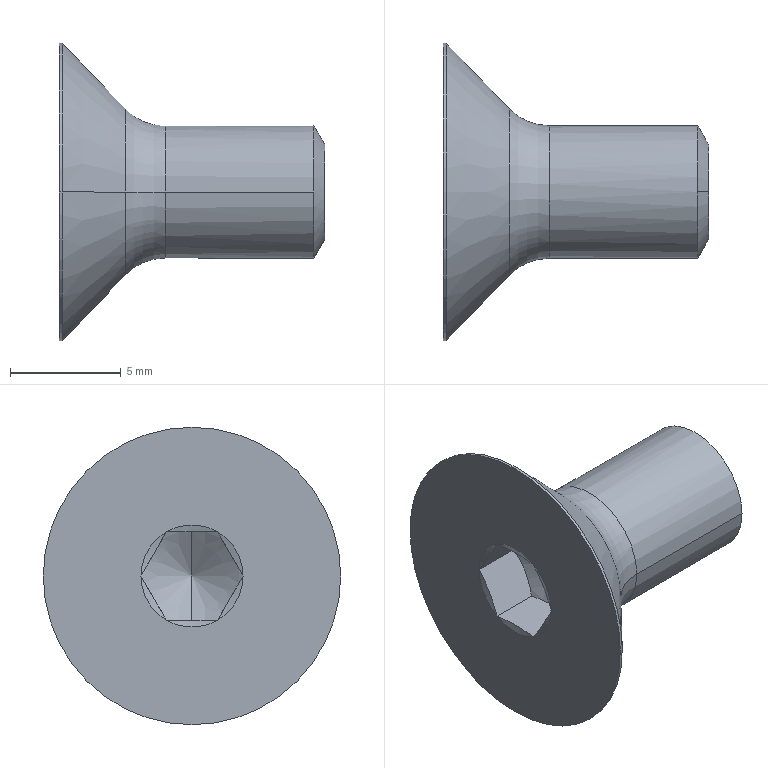Part | SolidWorks | features RevCut 2, Revolution 2, Cut 1, LPattern 1, RefAxis 1 | 1 solid | 26 faces | box 12 x 13.44 x 13.44 mm | volume 493.143 mm3 | cone 12 | plane 8 | cylinder 4 | torus 2 | commonest cylinder face diameters 6 x2 13.44 x2
STEP:
#1=CARTESIAN_POINT('',(0.,0.,2.134));
#2=VERTEX_POINT('',#1);
#3=CARTESIAN_POINT('',(0.,0.,-2.134));
#4=VERTEX_POINT('',#3);
#5=CARTESIAN_POINT('',(0.,0.,0.));
#6=DIRECTION('',(-1.,0.,0.));
#7=DIRECTION('',(0.,0.,1.));
#8=AXIS2_PLACEMENT_3D('',#5,#6,#7);
#9=CIRCLE('',#8,2.134);
#10=EDGE_CURVE('',#2,#4,#9,.T.);
#11=ORIENTED_EDGE('',*,*,#10,.T.);
#12=CARTESIAN_POINT('',(-0.5,0.,-3.));
#13=VERTEX_POINT('',#12);
#14=CARTESIAN_POINT('',(-0.5,0.,-3.));
#15=DIRECTION('',(-0.5,0.,-0.866));
#16=VECTOR('',#15,1000.);
#17=LINE('',#14,#16);
#18=EDGE_CURVE('',#4,#13,#17,.T.);
#19=ORIENTED_EDGE('',*,*,#18,.T.);
#20=CARTESIAN_POINT('',(-0.5,3.,0.));
#21=VERTEX_POINT('',#20);
#22=CARTESIAN_POINT('',(-0.5,0.,0.));
#23=DIRECTION('',(-1.,0.,0.));
#24=DIRECTION('',(0.,0.,1.));
#25=AXIS2_PLACEMENT_3D('',#22,#23,#24);
#26=CIRCLE('',#25,3.);
#27=EDGE_CURVE('',#21,#13,#26,.T.);
#28=ORIENTED_EDGE('',*,*,#27,.F.);
#29=CARTESIAN_POINT('',(-0.5,0.,3.));
#30=VERTEX_POINT('',#29);
#31=CARTESIAN_POINT('',(-0.5,0.,0.));
#32=DIRECTION('',(-1.,0.,0.));
#33=DIRECTION('',(0.,0.,1.));
#34=AXIS2_PLACEMENT_3D('',#31,#32,#33);
#35=CIRCLE('',#34,3.);
#36=EDGE_CURVE('',#30,#21,#35,.T.);
#37=ORIENTED_EDGE('',*,*,#36,.F.);
#38=CARTESIAN_POINT('',(-0.5,0.,3.));
#39=DIRECTION('',(-0.5,0.,0.866));
#40=VECTOR('',#39,1000.);
#41=LINE('',#38,#40);
#42=EDGE_CURVE('',#2,#30,#41,.T.);
#43=ORIENTED_EDGE('',*,*,#42,.F.);
#44=EDGE_LOOP('',(#11,#19,#28,#37,#43));
#45=FACE_OUTER_BOUND('',#44,.T.);
#46=CARTESIAN_POINT('',(-0.5,0.,0.));
#47=DIRECTION('',(-1.,0.,0.));
#48=DIRECTION('',(0.,0.,1.));
#49=AXIS2_PLACEMENT_3D('',#46,#47,#48);
#50=CONICAL_SURFACE('',#49,3.,1.047);
#51=ADVANCED_FACE('',(#45),#50,.T.);
#52=CARTESIAN_POINT('',(-8.467,0.,0.));
#53=VERTEX_POINT('',#52);
#54=CARTESIAN_POINT('',(-9.621,0.,2.));
#55=VERTEX_POINT('',#54);
#56=CARTESIAN_POINT('',(-9.8,0.,2.309));
#57=DIRECTION('',(-0.5,0.,0.866));
#58=VECTOR('',#57,1000.);
#59=LINE('',#56,#58);
#60=EDGE_CURVE('',#53,#55,#59,.T.);
#61=ORIENTED_EDGE('',*,*,#60,.F.);
#62=CARTESIAN_POINT('',(-9.621,0.,-2.));
#63=VERTEX_POINT('',#62);
#64=CARTESIAN_POINT('',(-9.8,0.,-2.309));
#65=DIRECTION('',(-0.5,0.,-0.866));
#66=VECTOR('',#65,1000.);
#67=LINE('',#64,#66);
#68=EDGE_CURVE('',#53,#63,#67,.T.);
#69=ORIENTED_EDGE('',*,*,#68,.T.);
#70=CARTESIAN_POINT('',(-9.8,-1.155,-2.));
#71=VERTEX_POINT('',#70);
#72=CARTESIAN_POINT('',(-9.621,0.,-2.));
#73=CARTESIAN_POINT('',(-9.621,-0.1949,-2.));
#74=CARTESIAN_POINT('',(-9.638,-0.3888,-2.));
#75=CARTESIAN_POINT('',(-9.7,-0.7748,-2.));
#76=CARTESIAN_POINT('',(-9.746,-0.9671,-2.));
#77=CARTESIAN_POINT('',(-9.8,-1.155,-2.));
#78=B_SPLINE_CURVE_WITH_KNOTS('',3,(#72,#73,#74,#75,#76,#77),.UNSPECIFIED.,.F.,.F.,(4,2,4),(0.007354,0.007938,0.008523),.UNSPECIFIED.);
#79=EDGE_CURVE('',#63,#71,#78,.T.);
#80=ORIENTED_EDGE('',*,*,#79,.T.);
#81=CARTESIAN_POINT('',(-9.8,-2.309,0.));
#82=VERTEX_POINT('',#81);
#83=CARTESIAN_POINT('',(-9.8,-1.155,-2.));
#84=CARTESIAN_POINT('',(-9.691,-1.343,-1.673));
#85=CARTESIAN_POINT('',(-9.622,-1.535,-1.342));
#86=CARTESIAN_POINT('',(-9.621,-1.829,-0.8319));
#87=CARTESIAN_POINT('',(-9.638,-1.927,-0.662));
#88=CARTESIAN_POINT('',(-9.701,-2.12,-0.3283));
#89=CARTESIAN_POINT('',(-9.746,-2.215,-0.1635));
#90=CARTESIAN_POINT('',(-9.8,-2.309,0.));
#91=B_SPLINE_CURVE_WITH_KNOTS('',3,(#83,#84,#85,#86,#87,#88,#89,#90),.UNSPECIFIED.,.F.,.F.,(4,2,2,4),(0.000000238,0.001166,0.00175,0.002333),.UNSPECIFIED.);
#92=EDGE_CURVE('',#71,#82,#91,.T.);
#93=ORIENTED_EDGE('',*,*,#92,.T.);
#94=CARTESIAN_POINT('',(-9.8,-1.155,2.));
#95=VERTEX_POINT('',#94);
#96=CARTESIAN_POINT('',(-9.8,-2.309,0.));
#97=CARTESIAN_POINT('',(-9.691,-2.121,0.3266));
#98=CARTESIAN_POINT('',(-9.622,-1.929,0.658));
#99=CARTESIAN_POINT('',(-9.621,-1.635,1.168));
#100=CARTESIAN_POINT('',(-9.638,-1.537,1.338));
#101=CARTESIAN_POINT('',(-9.701,-1.344,1.672));
#102=CARTESIAN_POINT('',(-9.746,-1.249,1.837));
#103=CARTESIAN_POINT('',(-9.8,-1.155,2.));
#104=B_SPLINE_CURVE_WITH_KNOTS('',3,(#96,#97,#98,#99,#100,#101,#102,#103),.UNSPECIFIED.,.F.,.F.,(4,2,2,4),(0.000000238,0.001166,0.00175,0.002333),.UNSPECIFIED.);
#105=EDGE_CURVE('',#82,#95,#104,.T.);
#106=ORIENTED_EDGE('',*,*,#105,.T.);
#107=CARTESIAN_POINT('',(-9.8,-1.155,2.));
#108=CARTESIAN_POINT('',(-9.746,-0.9671,2.));
#109=CARTESIAN_POINT('',(-9.7,-0.7748,2.));
#110=CARTESIAN_POINT('',(-9.638,-0.3888,2.));
#111=CARTESIAN_POINT('',(-9.621,-0.1949,2.));
#112=CARTESIAN_POINT('',(-9.621,0.,2.));
#113=B_SPLINE_CURVE_WITH_KNOTS('',3,(#107,#108,#109,#110,#111,#112),.UNSPECIFIED.,.F.,.F.,(4,2,4),(0.00198,0.002564,0.003147),.UNSPECIFIED.);
#114=EDGE_CURVE('',#95,#55,#113,.T.);
#115=ORIENTED_EDGE('',*,*,#114,.T.);
#116=EDGE_LOOP('',(#61,#69,#80,#93,#106,#115));
#117=FACE_OUTER_BOUND('',#116,.T.);
#118=CARTESIAN_POINT('',(-9.8,0.,0.));
#119=DIRECTION('',(-1.,0.,0.));
#120=DIRECTION('',(0.,0.,1.));
#121=AXIS2_PLACEMENT_3D('',#118,#119,#120);
#122=CONICAL_SURFACE('',#121,2.309,1.047);
#123=ADVANCED_FACE('',(#117),#122,.F.);
#124=CARTESIAN_POINT('',(-7.219,-3.,0.));
#125=VERTEX_POINT('',#124);
#126=CARTESIAN_POINT('',(-7.219,3.,0.));
#127=VERTEX_POINT('',#126);
#128=CARTESIAN_POINT('',(-7.219,0.,0.));
#129=DIRECTION('',(1.,0.,0.));
#130=DIRECTION('',(0.,1.,0.));
#131=AXIS2_PLACEMENT_3D('',#128,#129,#130);
#132=CIRCLE('',#131,3.);
#133=EDGE_CURVE('',#125,#127,#132,.T.);
#134=ORIENTED_EDGE('',*,*,#133,.F.);
#135=CARTESIAN_POINT('',(-9.017,-3.763,0.));
#136=VERTEX_POINT('',#135);
#137=CARTESIAN_POINT('',(-7.219,-5.5,0.));
#138=DIRECTION('',(0.,0.,1.));
#139=DIRECTION('',(0.,-1.,0.));
#140=AXIS2_PLACEMENT_3D('',#137,#138,#139);
#141=CIRCLE('',#140,2.5);
#142=EDGE_CURVE('',#125,#136,#141,.T.);
#143=ORIENTED_EDGE('',*,*,#142,.T.);
#144=CARTESIAN_POINT('',(-9.017,3.763,0.));
#145=VERTEX_POINT('',#144);
#146=CARTESIAN_POINT('',(-9.017,0.,0.));
#147=DIRECTION('',(1.,0.,0.));
#148=DIRECTION('',(0.,1.,0.));
#149=AXIS2_PLACEMENT_3D('',#146,#147,#148);
#150=CIRCLE('',#149,3.763);
#151=EDGE_CURVE('',#136,#145,#150,.T.);
#152=ORIENTED_EDGE('',*,*,#151,.T.);
#153=CARTESIAN_POINT('',(-7.219,5.5,0.));
#154=DIRECTION('',(0.,0.,-1.));
#155=DIRECTION('',(-1.,0.,0.));
#156=AXIS2_PLACEMENT_3D('',#153,#154,#155);
#157=CIRCLE('',#156,2.5);
#158=EDGE_CURVE('',#127,#145,#157,.T.);
#159=ORIENTED_EDGE('',*,*,#158,.F.);
#160=EDGE_LOOP('',(#134,#143,#152,#159));
#161=FACE_OUTER_BOUND('',#160,.T.);
#162=CARTESIAN_POINT('',(-7.219,0.,0.));
#163=DIRECTION('',(1.,0.,0.));
#164=DIRECTION('',(0.,1.,0.));
#165=AXIS2_PLACEMENT_3D('',#162,#163,#164);
#166=TOROIDAL_SURFACE('',#165,5.5,2.5);
#167=ADVANCED_FACE('',(#161),#166,.F.);
#168=CARTESIAN_POINT('',(-9.017,0.,0.));
#169=DIRECTION('',(1.,0.,0.));
#170=DIRECTION('',(0.,1.,0.));
#171=AXIS2_PLACEMENT_3D('',#168,#169,#170);
#172=CIRCLE('',#171,3.763);
#173=EDGE_CURVE('',#145,#136,#172,.T.);
#174=ORIENTED_EDGE('',*,*,#173,.F.);
#175=CARTESIAN_POINT('',(-11.872,6.72,0.));
#176=VERTEX_POINT('',#175);
#177=CARTESIAN_POINT('',(-9.017,3.763,0.));
#178=DIRECTION('',(-0.6947,0.7193,0.));
#179=VECTOR('',#178,1000.);
#180=LINE('',#177,#179);
#181=EDGE_CURVE('',#145,#176,#180,.T.);
#182=ORIENTED_EDGE('',*,*,#181,.T.);
#183=CARTESIAN_POINT('',(-11.872,-6.72,0.));
#184=VERTEX_POINT('',#183);
#185=CARTESIAN_POINT('',(-11.872,0.,0.));
#186=DIRECTION('',(1.,0.,0.));
#187=DIRECTION('',(0.,1.,0.));
#188=AXIS2_PLACEMENT_3D('',#185,#186,#187);
#189=CIRCLE('',#188,6.72);
#190=EDGE_CURVE('',#176,#184,#189,.T.);
#191=ORIENTED_EDGE('',*,*,#190,.T.);
#192=CARTESIAN_POINT('',(-9.017,-3.763,0.));
#193=DIRECTION('',(-0.6947,-0.7193,0.));
#194=VECTOR('',#193,1000.);
#195=LINE('',#192,#194);
#196=EDGE_CURVE('',#136,#184,#195,.T.);
#197=ORIENTED_EDGE('',*,*,#196,.F.);
#198=EDGE_LOOP('',(#174,#182,#191,#197));
#199=FACE_OUTER_BOUND('',#198,.T.);
#200=CARTESIAN_POINT('',(-9.017,0.,0.));
#201=DIRECTION('',(-1.,0.,0.));
#202=DIRECTION('',(0.,-1.,0.));
#203=AXIS2_PLACEMENT_3D('',#200,#201,#202);
#204=CONICAL_SURFACE('',#203,3.763,0.8029);
#205=ADVANCED_FACE('',(#199),#204,.T.);
#206=CARTESIAN_POINT('',(-12.,6.72,0.));
#207=VERTEX_POINT('',#206);
#208=CARTESIAN_POINT('',(-12.,-6.72,0.));
#209=VERTEX_POINT('',#208);
#210=CARTESIAN_POINT('',(-12.,0.,0.));
#211=DIRECTION('',(1.,0.,0.));
#212=DIRECTION('',(0.,1.,0.));
#213=AXIS2_PLACEMENT_3D('',#210,#211,#212);
#214=CIRCLE('',#213,6.72);
#215=EDGE_CURVE('',#207,#209,#214,.T.);
#216=ORIENTED_EDGE('',*,*,#215,.T.);
#217=CARTESIAN_POINT('',(0.,-6.72,0.));
#218=DIRECTION('',(1.,0.,0.));
#219=VECTOR('',#218,1000.);
#220=LINE('',#217,#219);
#221=EDGE_CURVE('',#209,#184,#220,.T.);
#222=ORIENTED_EDGE('',*,*,#221,.T.);
#223=ORIENTED_EDGE('',*,*,#190,.F.);
#224=CARTESIAN_POINT('',(0.,6.72,0.));
#225=DIRECTION('',(1.,0.,0.));
#226=VECTOR('',#225,1000.);
#227=LINE('',#224,#226);
#228=EDGE_CURVE('',#207,#176,#227,.T.);
#229=ORIENTED_EDGE('',*,*,#228,.F.);
#230=EDGE_LOOP('',(#216,#222,#223,#229));
#231=FACE_OUTER_BOUND('',#230,.T.);
#232=CARTESIAN_POINT('',(0.,0.,0.));
#233=DIRECTION('',(1.,0.,0.));
#234=DIRECTION('',(0.,1.,0.));
#235=AXIS2_PLACEMENT_3D('',#232,#233,#234);
#236=CYLINDRICAL_SURFACE('',#235,6.72);
#237=ADVANCED_FACE('',(#231),#236,.T.);
#238=CARTESIAN_POINT('',(-7.219,0.,0.));
#239=DIRECTION('',(1.,0.,0.));
#240=DIRECTION('',(0.,1.,0.));
#241=AXIS2_PLACEMENT_3D('',#238,#239,#240);
#242=CIRCLE('',#241,3.);
#243=EDGE_CURVE('',#127,#125,#242,.T.);
#244=ORIENTED_EDGE('',*,*,#243,.T.);
#245=CARTESIAN_POINT('',(-0.5,-3.,0.));
#246=VERTEX_POINT('',#245);
#247=CARTESIAN_POINT('',(0.,-3.,0.));
#248=DIRECTION('',(1.,0.,0.));
#249=VECTOR('',#248,1000.);
#250=LINE('',#247,#249);
#251=EDGE_CURVE('',#125,#246,#250,.T.);
#252=ORIENTED_EDGE('',*,*,#251,.T.);
#253=CARTESIAN_POINT('',(-0.5,0.,0.));
#254=DIRECTION('',(-1.,0.,0.));
#255=DIRECTION('',(0.,0.,1.));
#256=AXIS2_PLACEMENT_3D('',#253,#254,#255);
#257=CIRCLE('',#256,3.);
#258=EDGE_CURVE('',#246,#30,#257,.T.);
#259=ORIENTED_EDGE('',*,*,#258,.T.);
#260=ORIENTED_EDGE('',*,*,#36,.T.);
#261=CARTESIAN_POINT('',(0.,3.,0.));
#262=DIRECTION('',(1.,0.,0.));
#263=VECTOR('',#262,1000.);
#264=LINE('',#261,#263);
#265=EDGE_CURVE('',#127,#21,#264,.T.);
#266=ORIENTED_EDGE('',*,*,#265,.F.);
#267=EDGE_LOOP('',(#244,#252,#259,#260,#266));
#268=FACE_OUTER_BOUND('',#267,.T.);
#269=CARTESIAN_POINT('',(0.,0.,0.));
#270=DIRECTION('',(1.,0.,0.));
#271=DIRECTION('',(0.,1.,0.));
#272=AXIS2_PLACEMENT_3D('',#269,#270,#271);
#273=CYLINDRICAL_SURFACE('',#272,3.);
#274=ADVANCED_FACE('',(#268),#273,.T.);
#275=ORIENTED_EDGE('',*,*,#251,.F.);
#276=ORIENTED_EDGE('',*,*,#133,.T.);
#277=ORIENTED_EDGE('',*,*,#265,.T.);
#278=ORIENTED_EDGE('',*,*,#27,.T.);
#279=CARTESIAN_POINT('',(-0.5,0.,0.));
#280=DIRECTION('',(-1.,0.,0.));
#281=DIRECTION('',(0.,0.,1.));
#282=AXIS2_PLACEMENT_3D('',#279,#280,#281);
#283=CIRCLE('',#282,3.);
#284=EDGE_CURVE('',#13,#246,#283,.T.);
#285=ORIENTED_EDGE('',*,*,#284,.T.);
#286=EDGE_LOOP('',(#275,#276,#277,#278,#285));
#287=FACE_OUTER_BOUND('',#286,.T.);
#288=CARTESIAN_POINT('',(0.,0.,0.));
#289=DIRECTION('',(1.,0.,0.));
#290=DIRECTION('',(0.,1.,0.));
#291=AXIS2_PLACEMENT_3D('',#288,#289,#290);
#292=CYLINDRICAL_SURFACE('',#291,3.);
#293=ADVANCED_FACE('',(#287),#292,.T.);
#294=ORIENTED_EDGE('',*,*,#215,.F.);
#295=CARTESIAN_POINT('',(-12.,0.,0.));
#296=DIRECTION('',(1.,0.,0.));
#297=DIRECTION('',(0.,1.,0.));
#298=AXIS2_PLACEMENT_3D('',#295,#296,#297);
#299=CIRCLE('',#298,6.72);
#300=EDGE_CURVE('',#209,#207,#299,.T.);
#301=ORIENTED_EDGE('',*,*,#300,.F.);
#302=EDGE_LOOP('',(#294,#301));
#303=FACE_OUTER_BOUND('',#302,.T.);
#304=CARTESIAN_POINT('',(-12.,-2.309,0.));
#305=VERTEX_POINT('',#304);
#306=CARTESIAN_POINT('',(-12.,-1.155,2.));
#307=VERTEX_POINT('',#306);
#308=CARTESIAN_POINT('',(-12.,0.,0.));
#309=DIRECTION('',(-1.,0.,0.));
#310=DIRECTION('',(0.,-1.,0.));
#311=AXIS2_PLACEMENT_3D('',#308,#309,#310);
#312=CIRCLE('',#311,2.309);
#313=EDGE_CURVE('',#305,#307,#312,.T.);
#314=ORIENTED_EDGE('',*,*,#313,.F.);
#315=CARTESIAN_POINT('',(-12.,-1.155,-2.));
#316=VERTEX_POINT('',#315);
#317=CARTESIAN_POINT('',(-12.,0.,0.));
#318=DIRECTION('',(1.,0.,0.));
#319=DIRECTION('',(0.,-1.,0.));
#320=AXIS2_PLACEMENT_3D('',#317,#318,#319);
#321=CIRCLE('',#320,2.309);
#322=EDGE_CURVE('',#305,#316,#321,.T.);
#323=ORIENTED_EDGE('',*,*,#322,.T.);
#324=CARTESIAN_POINT('',(-12.,1.155,-2.));
#325=VERTEX_POINT('',#324);
#326=CARTESIAN_POINT('',(-12.,0.,0.));
#327=DIRECTION('',(1.,0.,0.));
#328=DIRECTION('',(0.,-1.,0.));
#329=AXIS2_PLACEMENT_3D('',#326,#327,#328);
#330=CIRCLE('',#329,2.309);
#331=EDGE_CURVE('',#316,#325,#330,.T.);
#332=ORIENTED_EDGE('',*,*,#331,.T.);
#333=CARTESIAN_POINT('',(-12.,2.309,0.));
#334=VERTEX_POINT('',#333);
#335=CARTESIAN_POINT('',(-12.,0.,0.));
#336=DIRECTION('',(1.,0.,0.));
#337=DIRECTION('',(0.,-1.,0.));
#338=AXIS2_PLACEMENT_3D('',#335,#336,#337);
#339=CIRCLE('',#338,2.309);
#340=EDGE_CURVE('',#325,#334,#339,.T.);
#341=ORIENTED_EDGE('',*,*,#340,.T.);
#342=CARTESIAN_POINT('',(-12.,1.155,2.));
#343=VERTEX_POINT('',#342);
#344=CARTESIAN_POINT('',(-12.,0.,0.));
#345=DIRECTION('',(1.,0.,0.));
#346=DIRECTION('',(0.,-1.,0.));
#347=AXIS2_PLACEMENT_3D('',#344,#345,#346);
#348=CIRCLE('',#347,2.309);
#349=EDGE_CURVE('',#334,#343,#348,.T.);
#350=ORIENTED_EDGE('',*,*,#349,.T.);
#351=CARTESIAN_POINT('',(-12.,0.,0.));
#352=DIRECTION('',(1.,0.,0.));
#353=DIRECTION('',(0.,-1.,0.));
#354=AXIS2_PLACEMENT_3D('',#351,#352,#353);
#355=CIRCLE('',#354,2.309);
#356=EDGE_CURVE('',#343,#307,#355,.T.);
#357=ORIENTED_EDGE('',*,*,#356,.T.);
#358=EDGE_LOOP('',(#314,#323,#332,#341,#350,#357));
#359=FACE_BOUND('',#358,.T.);
#360=CARTESIAN_POINT('',(-12.,6.72,0.));
#361=DIRECTION('',(-1.,0.,0.));
#362=DIRECTION('',(0.,-1.,0.));
#363=AXIS2_PLACEMENT_3D('',#360,#361,#362);
#364=PLANE('',#363);
#365=ADVANCED_FACE('',(#303,#359),#364,.T.);
#366=ORIENTED_EDGE('',*,*,#221,.F.);
#367=ORIENTED_EDGE('',*,*,#300,.T.);
#368=ORIENTED_EDGE('',*,*,#228,.T.);
#369=CARTESIAN_POINT('',(-11.872,0.,0.));
#370=DIRECTION('',(1.,0.,0.));
#371=DIRECTION('',(0.,1.,0.));
#372=AXIS2_PLACEMENT_3D('',#369,#370,#371);
#373=CIRCLE('',#372,6.72);
#374=EDGE_CURVE('',#184,#176,#373,.T.);
#375=ORIENTED_EDGE('',*,*,#374,.F.);
#376=EDGE_LOOP('',(#366,#367,#368,#375));
#377=FACE_OUTER_BOUND('',#376,.T.);
#378=CARTESIAN_POINT('',(0.,0.,0.));
#379=DIRECTION('',(1.,0.,0.));
#380=DIRECTION('',(0.,1.,0.));
#381=AXIS2_PLACEMENT_3D('',#378,#379,#380);
#382=CYLINDRICAL_SURFACE('',#381,6.72);
#383=ADVANCED_FACE('',(#377),#382,.T.);
#384=ORIENTED_EDGE('',*,*,#181,.F.);
#385=ORIENTED_EDGE('',*,*,#151,.F.);
#386=ORIENTED_EDGE('',*,*,#196,.T.);
#387=ORIENTED_EDGE('',*,*,#374,.T.);
#388=EDGE_LOOP('',(#384,#385,#386,#387));
#389=FACE_OUTER_BOUND('',#388,.T.);
#390=CARTESIAN_POINT('',(-9.017,0.,0.));
#391=DIRECTION('',(-1.,0.,0.));
#392=DIRECTION('',(0.,-1.,0.));
#393=AXIS2_PLACEMENT_3D('',#390,#391,#392);
#394=CONICAL_SURFACE('',#393,3.763,0.8029);
#395=ADVANCED_FACE('',(#389),#394,.T.);
#396=ORIENTED_EDGE('',*,*,#142,.F.);
#397=ORIENTED_EDGE('',*,*,#243,.F.);
#398=ORIENTED_EDGE('',*,*,#158,.T.);
#399=ORIENTED_EDGE('',*,*,#173,.T.);
#400=EDGE_LOOP('',(#396,#397,#398,#399));
#401=FACE_OUTER_BOUND('',#400,.T.);
#402=CARTESIAN_POINT('',(-7.219,0.,0.));
#403=DIRECTION('',(1.,0.,0.));
#404=DIRECTION('',(0.,1.,0.));
#405=AXIS2_PLACEMENT_3D('',#402,#403,#404);
#406=TOROIDAL_SURFACE('',#405,5.5,2.5);
#407=ADVANCED_FACE('',(#401),#406,.F.);
#408=CARTESIAN_POINT('',(-12.,-1.155,2.));
#409=CARTESIAN_POINT('',(-11.947,-1.347,1.667));
#410=CARTESIAN_POINT('',(-11.882,-1.732,1.));
#411=CARTESIAN_POINT('',(-11.947,-2.117,0.3333));
#412=CARTESIAN_POINT('',(-12.,-2.309,0.));
#413=B_SPLINE_CURVE_WITH_KNOTS('',3,(#408,#409,#410,#411,#412),.UNSPECIFIED.,.F.,.F.,(4,1,4),(0.000000231,0.001155,0.00231),.UNSPECIFIED.);
#414=EDGE_CURVE('',#307,#305,#413,.T.);
#415=ORIENTED_EDGE('',*,*,#414,.T.);
#416=ORIENTED_EDGE('',*,*,#313,.T.);
#417=EDGE_LOOP('',(#415,#416));
#418=FACE_OUTER_BOUND('',#417,.T.);
#419=CARTESIAN_POINT('',(-1011.362,0.,0.));
#420=DIRECTION('',(-1.,0.,0.));
#421=DIRECTION('',(0.,-1.,0.));
#422=AXIS2_PLACEMENT_3D('',#419,#420,#421);
#423=CONICAL_SURFACE('',#422,3619.751,1.301);
#424=ADVANCED_FACE('',(#418),#423,.F.);
#425=CARTESIAN_POINT('',(-12.,1.155,2.));
#426=CARTESIAN_POINT('',(-11.947,0.7714,2.));
#427=CARTESIAN_POINT('',(-11.915,0.3874,2.));
#428=CARTESIAN_POINT('',(-11.914,-0.3828,2.));
#429=CARTESIAN_POINT('',(-11.947,-0.7704,2.));
#430=CARTESIAN_POINT('',(-12.,-1.155,2.));
#431=B_SPLINE_CURVE_WITH_KNOTS('',3,(#425,#426,#427,#428,#429,#430),.UNSPECIFIED.,.F.,.F.,(4,2,4),(0.004828,0.005989,0.007149),.UNSPECIFIED.);
#432=EDGE_CURVE('',#343,#307,#431,.T.);
#433=ORIENTED_EDGE('',*,*,#432,.T.);
#434=ORIENTED_EDGE('',*,*,#356,.F.);
#435=EDGE_LOOP('',(#433,#434));
#436=FACE_OUTER_BOUND('',#435,.T.);
#437=CARTESIAN_POINT('',(-1011.362,0.,0.));
#438=DIRECTION('',(-1.,0.,0.));
#439=DIRECTION('',(0.,-1.,0.));
#440=AXIS2_PLACEMENT_3D('',#437,#438,#439);
#441=CONICAL_SURFACE('',#440,3619.751,1.301);
#442=ADVANCED_FACE('',(#436),#441,.F.);
#443=CARTESIAN_POINT('',(-12.,2.309,0.));
#444=CARTESIAN_POINT('',(-11.947,2.117,0.3333));
#445=CARTESIAN_POINT('',(-11.882,1.732,1.));
#446=CARTESIAN_POINT('',(-11.947,1.347,1.667));
#447=CARTESIAN_POINT('',(-12.,1.155,2.));
#448=B_SPLINE_CURVE_WITH_KNOTS('',3,(#443,#444,#445,#446,#447),.UNSPECIFIED.,.F.,.F.,(4,1,4),(0.000000231,0.001155,0.00231),.UNSPECIFIED.);
#449=EDGE_CURVE('',#334,#343,#448,.T.);
#450=ORIENTED_EDGE('',*,*,#449,.T.);
#451=ORIENTED_EDGE('',*,*,#349,.F.);
#452=EDGE_LOOP('',(#450,#451));
#453=FACE_OUTER_BOUND('',#452,.T.);
#454=CARTESIAN_POINT('',(-1011.362,0.,0.));
#455=DIRECTION('',(-1.,0.,0.));
#456=DIRECTION('',(0.,-1.,0.));
#457=AXIS2_PLACEMENT_3D('',#454,#455,#456);
#458=CONICAL_SURFACE('',#457,3619.751,1.301);
#459=ADVANCED_FACE('',(#453),#458,.F.);
#460=CARTESIAN_POINT('',(-12.,1.155,-2.));
#461=CARTESIAN_POINT('',(-11.947,1.347,-1.667));
#462=CARTESIAN_POINT('',(-11.882,1.732,-1.));
#463=CARTESIAN_POINT('',(-11.947,2.117,-0.3333));
#464=CARTESIAN_POINT('',(-12.,2.309,0.));
#465=B_SPLINE_CURVE_WITH_KNOTS('',3,(#460,#461,#462,#463,#464),.UNSPECIFIED.,.F.,.F.,(4,1,4),(0.000000231,0.001155,0.00231),.UNSPECIFIED.);
#466=EDGE_CURVE('',#325,#334,#465,.T.);
#467=ORIENTED_EDGE('',*,*,#466,.T.);
#468=ORIENTED_EDGE('',*,*,#340,.F.);
#469=EDGE_LOOP('',(#467,#468));
#470=FACE_OUTER_BOUND('',#469,.T.);
#471=CARTESIAN_POINT('',(-1011.362,0.,0.));
#472=DIRECTION('',(-1.,0.,0.));
#473=DIRECTION('',(0.,-1.,0.));
#474=AXIS2_PLACEMENT_3D('',#471,#472,#473);
#475=CONICAL_SURFACE('',#474,3619.751,1.301);
#476=ADVANCED_FACE('',(#470),#475,.F.);
#477=CARTESIAN_POINT('',(-12.,-1.155,-2.));
#478=CARTESIAN_POINT('',(-11.947,-0.7704,-2.));
#479=CARTESIAN_POINT('',(-11.914,-0.3828,-2.));
#480=CARTESIAN_POINT('',(-11.915,0.3874,-2.));
#481=CARTESIAN_POINT('',(-11.947,0.7714,-2.));
#482=CARTESIAN_POINT('',(-12.,1.155,-2.));
#483=B_SPLINE_CURVE_WITH_KNOTS('',3,(#477,#478,#479,#480,#481,#482),.UNSPECIFIED.,.F.,.F.,(4,2,4),(0.001892,0.003055,0.004218),.UNSPECIFIED.);
#484=EDGE_CURVE('',#316,#325,#483,.T.);
#485=ORIENTED_EDGE('',*,*,#484,.T.);
#486=ORIENTED_EDGE('',*,*,#331,.F.);
#487=EDGE_LOOP('',(#485,#486));
#488=FACE_OUTER_BOUND('',#487,.T.);
#489=CARTESIAN_POINT('',(-1011.362,0.,0.));
#490=DIRECTION('',(-1.,0.,0.));
#491=DIRECTION('',(0.,-1.,0.));
#492=AXIS2_PLACEMENT_3D('',#489,#490,#491);
#493=CONICAL_SURFACE('',#492,3619.751,1.301);
#494=ADVANCED_FACE('',(#488),#493,.F.);
#495=CARTESIAN_POINT('',(-12.,-2.309,0.));
#496=CARTESIAN_POINT('',(-11.947,-2.117,-0.3333));
#497=CARTESIAN_POINT('',(-11.882,-1.732,-1.));
#498=CARTESIAN_POINT('',(-11.947,-1.347,-1.667));
#499=CARTESIAN_POINT('',(-12.,-1.155,-2.));
#500=B_SPLINE_CURVE_WITH_KNOTS('',3,(#495,#496,#497,#498,#499),.UNSPECIFIED.,.F.,.F.,(4,1,4),(0.000000231,0.001155,0.00231),.UNSPECIFIED.);
#501=EDGE_CURVE('',#305,#316,#500,.T.);
#502=ORIENTED_EDGE('',*,*,#501,.T.);
#503=ORIENTED_EDGE('',*,*,#322,.F.);
#504=EDGE_LOOP('',(#502,#503));
#505=FACE_OUTER_BOUND('',#504,.T.);
#506=CARTESIAN_POINT('',(-1011.362,0.,0.));
#507=DIRECTION('',(-1.,0.,0.));
#508=DIRECTION('',(0.,-1.,0.));
#509=AXIS2_PLACEMENT_3D('',#506,#507,#508);
#510=CONICAL_SURFACE('',#509,3619.751,1.301);
#511=ADVANCED_FACE('',(#505),#510,.F.);
#512=ORIENTED_EDGE('',*,*,#68,.F.);
#513=ORIENTED_EDGE('',*,*,#60,.T.);
#514=CARTESIAN_POINT('',(-9.8,1.155,2.));
#515=VERTEX_POINT('',#514);
#516=CARTESIAN_POINT('',(-9.621,0.,2.));
#517=CARTESIAN_POINT('',(-9.621,0.195,2.));
#518=CARTESIAN_POINT('',(-9.639,0.3927,2.));
#519=CARTESIAN_POINT('',(-9.701,0.7788,2.));
#520=CARTESIAN_POINT('',(-9.746,0.968,2.));
#521=CARTESIAN_POINT('',(-9.8,1.155,2.));
#522=B_SPLINE_CURVE_WITH_KNOTS('',3,(#516,#517,#518,#519,#520,#521),.UNSPECIFIED.,.F.,.F.,(4,2,4),(0.003147,0.003731,0.004315),.UNSPECIFIED.);
#523=EDGE_CURVE('',#55,#515,#522,.T.);
#524=ORIENTED_EDGE('',*,*,#523,.T.);
#525=CARTESIAN_POINT('',(-9.8,2.309,0.));
#526=VERTEX_POINT('',#525);
#527=CARTESIAN_POINT('',(-9.8,1.155,2.));
#528=CARTESIAN_POINT('',(-9.691,1.343,1.673));
#529=CARTESIAN_POINT('',(-9.622,1.535,1.342));
#530=CARTESIAN_POINT('',(-9.621,1.829,0.8319));
#531=CARTESIAN_POINT('',(-9.638,1.927,0.662));
#532=CARTESIAN_POINT('',(-9.701,2.12,0.3283));
#533=CARTESIAN_POINT('',(-9.746,2.215,0.1635));
#534=CARTESIAN_POINT('',(-9.8,2.309,0.));
#535=B_SPLINE_CURVE_WITH_KNOTS('',3,(#527,#528,#529,#530,#531,#532,#533,#534),.UNSPECIFIED.,.F.,.F.,(4,2,2,4),(0.000000238,0.001166,0.00175,0.002333),.UNSPECIFIED.);
#536=EDGE_CURVE('',#515,#526,#535,.T.);
#537=ORIENTED_EDGE('',*,*,#536,.T.);
#538=CARTESIAN_POINT('',(-9.8,1.155,-2.));
#539=VERTEX_POINT('',#538);
#540=CARTESIAN_POINT('',(-9.8,2.309,0.));
#541=CARTESIAN_POINT('',(-9.691,2.121,-0.3266));
#542=CARTESIAN_POINT('',(-9.622,1.929,-0.658));
#543=CARTESIAN_POINT('',(-9.621,1.635,-1.168));
#544=CARTESIAN_POINT('',(-9.638,1.537,-1.338));
#545=CARTESIAN_POINT('',(-9.701,1.344,-1.672));
#546=CARTESIAN_POINT('',(-9.746,1.249,-1.837));
#547=CARTESIAN_POINT('',(-9.8,1.155,-2.));
#548=B_SPLINE_CURVE_WITH_KNOTS('',3,(#540,#541,#542,#543,#544,#545,#546,#547),.UNSPECIFIED.,.F.,.F.,(4,2,2,4),(0.000000238,0.001166,0.00175,0.002333),.UNSPECIFIED.);
#549=EDGE_CURVE('',#526,#539,#548,.T.);
#550=ORIENTED_EDGE('',*,*,#549,.T.);
#551=CARTESIAN_POINT('',(-9.8,1.155,-2.));
#552=CARTESIAN_POINT('',(-9.746,0.968,-2.));
#553=CARTESIAN_POINT('',(-9.701,0.7788,-2.));
#554=CARTESIAN_POINT('',(-9.639,0.3927,-2.));
#555=CARTESIAN_POINT('',(-9.621,0.195,-2.));
#556=CARTESIAN_POINT('',(-9.621,0.,-2.));
#557=B_SPLINE_CURVE_WITH_KNOTS('',3,(#551,#552,#553,#554,#555,#556),.UNSPECIFIED.,.F.,.F.,(4,2,4),(0.006185,0.006769,0.007354),.UNSPECIFIED.);
#558=EDGE_CURVE('',#539,#63,#557,.T.);
#559=ORIENTED_EDGE('',*,*,#558,.T.);
#560=EDGE_LOOP('',(#512,#513,#524,#537,#550,#559));
#561=FACE_OUTER_BOUND('',#560,.T.);
#562=CARTESIAN_POINT('',(-9.8,0.,0.));
#563=DIRECTION('',(-1.,0.,0.));
#564=DIRECTION('',(0.,0.,1.));
#565=AXIS2_PLACEMENT_3D('',#562,#563,#564);
#566=CONICAL_SURFACE('',#565,2.309,1.047);
#567=ADVANCED_FACE('',(#561),#566,.F.);
#568=ORIENTED_EDGE('',*,*,#466,.F.);
#569=CARTESIAN_POINT('',(-8.18,1.155,-2.));
#570=DIRECTION('',(-1.,0.,0.));
#571=VECTOR('',#570,1000.);
#572=LINE('',#569,#571);
#573=EDGE_CURVE('',#539,#325,#572,.T.);
#574=ORIENTED_EDGE('',*,*,#573,.F.);
#575=ORIENTED_EDGE('',*,*,#549,.F.);
#576=CARTESIAN_POINT('',(-8.18,2.309,0.));
#577=DIRECTION('',(-1.,0.,0.));
#578=VECTOR('',#577,1000.);
#579=LINE('',#576,#578);
#580=EDGE_CURVE('',#526,#334,#579,.T.);
#581=ORIENTED_EDGE('',*,*,#580,.T.);
#582=EDGE_LOOP('',(#568,#574,#575,#581));
#583=FACE_OUTER_BOUND('',#582,.T.);
#584=CARTESIAN_POINT('',(-8.18,2.309,0.));
#585=DIRECTION('',(0.,0.866,-0.5));
#586=DIRECTION('',(0.,0.5,0.866));
#587=AXIS2_PLACEMENT_3D('',#584,#585,#586);
#588=PLANE('',#587);
#589=ADVANCED_FACE('',(#583),#588,.F.);
#590=ORIENTED_EDGE('',*,*,#484,.F.);
#591=CARTESIAN_POINT('',(-8.18,-1.155,-2.));
#592=DIRECTION('',(-1.,0.,0.));
#593=VECTOR('',#592,1000.);
#594=LINE('',#591,#593);
#595=EDGE_CURVE('',#71,#316,#594,.T.);
#596=ORIENTED_EDGE('',*,*,#595,.F.);
#597=ORIENTED_EDGE('',*,*,#79,.F.);
#598=ORIENTED_EDGE('',*,*,#558,.F.);
#599=ORIENTED_EDGE('',*,*,#573,.T.);
#600=EDGE_LOOP('',(#590,#596,#597,#598,#599));
#601=FACE_OUTER_BOUND('',#600,.T.);
#602=CARTESIAN_POINT('',(-8.18,1.155,-2.));
#603=DIRECTION('',(0.,0.,-1.));
#604=DIRECTION('',(-1.,0.,0.));
#605=AXIS2_PLACEMENT_3D('',#602,#603,#604);
#606=PLANE('',#605);
#607=ADVANCED_FACE('',(#601),#606,.F.);
#608=ORIENTED_EDGE('',*,*,#501,.F.);
#609=CARTESIAN_POINT('',(-8.18,-2.309,0.));
#610=DIRECTION('',(-1.,0.,0.));
#611=VECTOR('',#610,1000.);
#612=LINE('',#609,#611);
#613=EDGE_CURVE('',#82,#305,#612,.T.);
#614=ORIENTED_EDGE('',*,*,#613,.F.);
#615=ORIENTED_EDGE('',*,*,#92,.F.);
#616=ORIENTED_EDGE('',*,*,#595,.T.);
#617=EDGE_LOOP('',(#608,#614,#615,#616));
#618=FACE_OUTER_BOUND('',#617,.T.);
#619=CARTESIAN_POINT('',(-8.18,-1.155,-2.));
#620=DIRECTION('',(0.,-0.866,-0.5));
#621=DIRECTION('',(0.,0.5,-0.866));
#622=AXIS2_PLACEMENT_3D('',#619,#620,#621);
#623=PLANE('',#622);
#624=ADVANCED_FACE('',(#618),#623,.F.);
#625=ORIENTED_EDGE('',*,*,#414,.F.);
#626=CARTESIAN_POINT('',(-8.18,-1.155,2.));
#627=DIRECTION('',(-1.,0.,0.));
#628=VECTOR('',#627,1000.);
#629=LINE('',#626,#628);
#630=EDGE_CURVE('',#95,#307,#629,.T.);
#631=ORIENTED_EDGE('',*,*,#630,.F.);
#632=ORIENTED_EDGE('',*,*,#105,.F.);
#633=ORIENTED_EDGE('',*,*,#613,.T.);
#634=EDGE_LOOP('',(#625,#631,#632,#633));
#635=FACE_OUTER_BOUND('',#634,.T.);
#636=CARTESIAN_POINT('',(-8.18,-2.309,0.));
#637=DIRECTION('',(0.,-0.866,0.5));
#638=DIRECTION('',(0.,-0.5,-0.866));
#639=AXIS2_PLACEMENT_3D('',#636,#637,#638);
#640=PLANE('',#639);
#641=ADVANCED_FACE('',(#635),#640,.F.);
#642=ORIENTED_EDGE('',*,*,#432,.F.);
#643=CARTESIAN_POINT('',(-8.18,1.155,2.));
#644=DIRECTION('',(-1.,0.,0.));
#645=VECTOR('',#644,1000.);
#646=LINE('',#643,#645);
#647=EDGE_CURVE('',#515,#343,#646,.T.);
#648=ORIENTED_EDGE('',*,*,#647,.F.);
#649=ORIENTED_EDGE('',*,*,#523,.F.);
#650=ORIENTED_EDGE('',*,*,#114,.F.);
#651=ORIENTED_EDGE('',*,*,#630,.T.);
#652=EDGE_LOOP('',(#642,#648,#649,#650,#651));
#653=FACE_OUTER_BOUND('',#652,.T.);
#654=CARTESIAN_POINT('',(-8.18,-1.155,2.));
#655=DIRECTION('',(0.,0.,1.));
#656=DIRECTION('',(0.,-1.,0.));
#657=AXIS2_PLACEMENT_3D('',#654,#655,#656);
#658=PLANE('',#657);
#659=ADVANCED_FACE('',(#653),#658,.F.);
#660=ORIENTED_EDGE('',*,*,#449,.F.);
#661=ORIENTED_EDGE('',*,*,#580,.F.);
#662=ORIENTED_EDGE('',*,*,#536,.F.);
#663=ORIENTED_EDGE('',*,*,#647,.T.);
#664=EDGE_LOOP('',(#660,#661,#662,#663));
#665=FACE_OUTER_BOUND('',#664,.T.);
#666=CARTESIAN_POINT('',(-8.18,1.155,2.));
#667=DIRECTION('',(0.,0.866,0.5));
#668=DIRECTION('',(0.,-0.5,0.866));
#669=AXIS2_PLACEMENT_3D('',#666,#667,#668);
#670=PLANE('',#669);
#671=ADVANCED_FACE('',(#665),#670,.F.);
#672=ORIENTED_EDGE('',*,*,#18,.F.);
#673=CARTESIAN_POINT('',(0.,0.,0.));
#674=DIRECTION('',(-1.,0.,0.));
#675=DIRECTION('',(0.,0.,1.));
#676=AXIS2_PLACEMENT_3D('',#673,#674,#675);
#677=CIRCLE('',#676,2.134);
#678=EDGE_CURVE('',#4,#2,#677,.T.);
#679=ORIENTED_EDGE('',*,*,#678,.T.);
#680=ORIENTED_EDGE('',*,*,#42,.T.);
#681=ORIENTED_EDGE('',*,*,#258,.F.);
#682=ORIENTED_EDGE('',*,*,#284,.F.);
#683=EDGE_LOOP('',(#672,#679,#680,#681,#682));
#684=FACE_OUTER_BOUND('',#683,.T.);
#685=CARTESIAN_POINT('',(-0.5,0.,0.));
#686=DIRECTION('',(-1.,0.,0.));
#687=DIRECTION('',(0.,0.,1.));
#688=AXIS2_PLACEMENT_3D('',#685,#686,#687);
#689=CONICAL_SURFACE('',#688,3.,1.047);
#690=ADVANCED_FACE('',(#684),#689,.T.);
#691=ORIENTED_EDGE('',*,*,#10,.F.);
#692=ORIENTED_EDGE('',*,*,#678,.F.);
#693=EDGE_LOOP('',(#691,#692));
#694=FACE_OUTER_BOUND('',#693,.T.);
#695=CARTESIAN_POINT('',(0.,0.,0.));
#696=DIRECTION('',(1.,0.,0.));
#697=DIRECTION('',(0.,1.,0.));
#698=AXIS2_PLACEMENT_3D('',#695,#696,#697);
#699=PLANE('',#698);
#700=ADVANCED_FACE('',(#694),#699,.T.);
#701=CLOSED_SHELL('',(#51,#123,#167,#205,#237,#274,#293,#365,#383,#395,#407,#424,#442,#459,#476,#494,#511,#567,#589,#607,#624,#641,#659,#671,#690,#700));
#702=MANIFOLD_SOLID_BREP('',#701);
#703=CARTESIAN_POINT('',(0.,0.,0.));
#704=DIRECTION('',(0.,0.,1.));
#705=DIRECTION('',(1.,0.,0.));
#706=AXIS2_PLACEMENT_3D('',#703,#704,#705);
#707=(LENGTH_UNIT()NAMED_UNIT(*)SI_UNIT(.MILLI.,.METRE.));
#708=UNCERTAINTY_MEASURE_WITH_UNIT(LENGTH_MEASURE(0.00001),#707,'','');
#709=(NAMED_UNIT(*)PLANE_ANGLE_UNIT()SI_UNIT($,.RADIAN.));
#710=(NAMED_UNIT(*)SI_UNIT($,.STERADIAN.)SOLID_ANGLE_UNIT());
#711=(GEOMETRIC_REPRESENTATION_CONTEXT(3)GLOBAL_UNCERTAINTY_ASSIGNED_CONTEXT((#708))GLOBAL_UNIT_ASSIGNED_CONTEXT((#707,#709,#710))REPRESENTATION_CONTEXT('',''));
#712=ADVANCED_BREP_SHAPE_REPRESENTATION('',(#702,#706),#711);